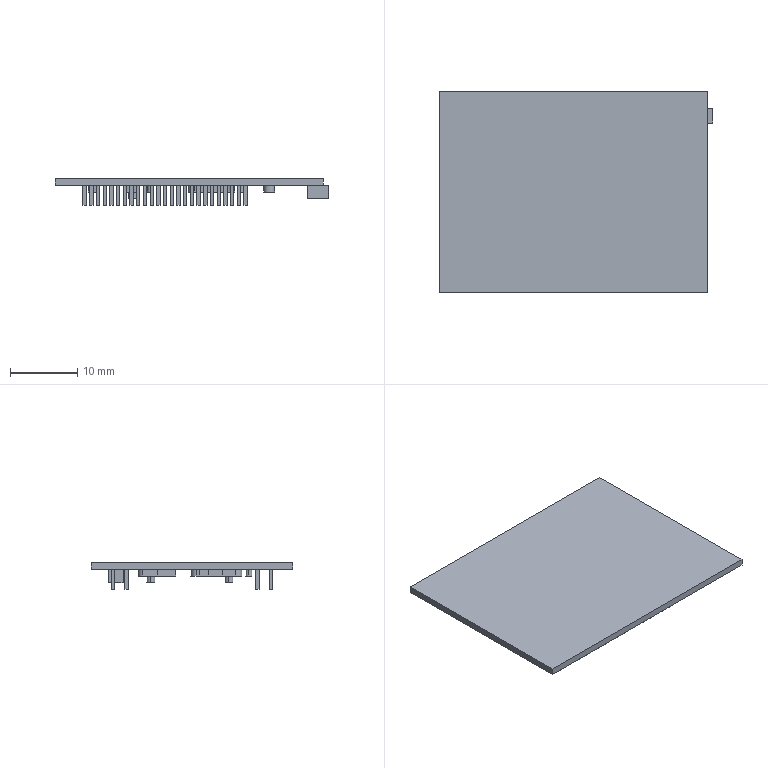Part | SolidWorks | features BaseBody 1 | 1 solid | 573 faces | box 40.811 x 30 x 4 mm | volume 1334 mm3 | plane 554 | cylinder 19 | commonest cylinder face diameters 0.924 x4 1.802 x3 0.971 x2 1.004 x2 1.151 x2 1.213 x2